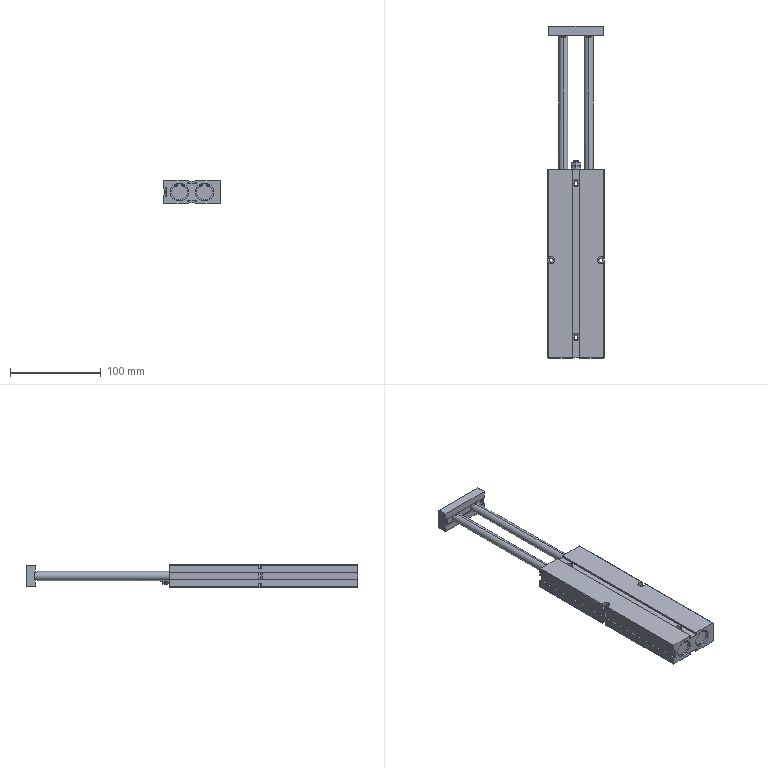Part | SolidWorks | 4 solids | 411 faces | box 62.3 x 366.5 x 25.2 mm | volume 245376 mm3 | cylinder 188 | plane 127 | cone 88 | torus 8 | commonest cylinder face diameters 0.4 x30 1.46 x16 3.5 x16 19.6 x16 17.5 x12 20 x12